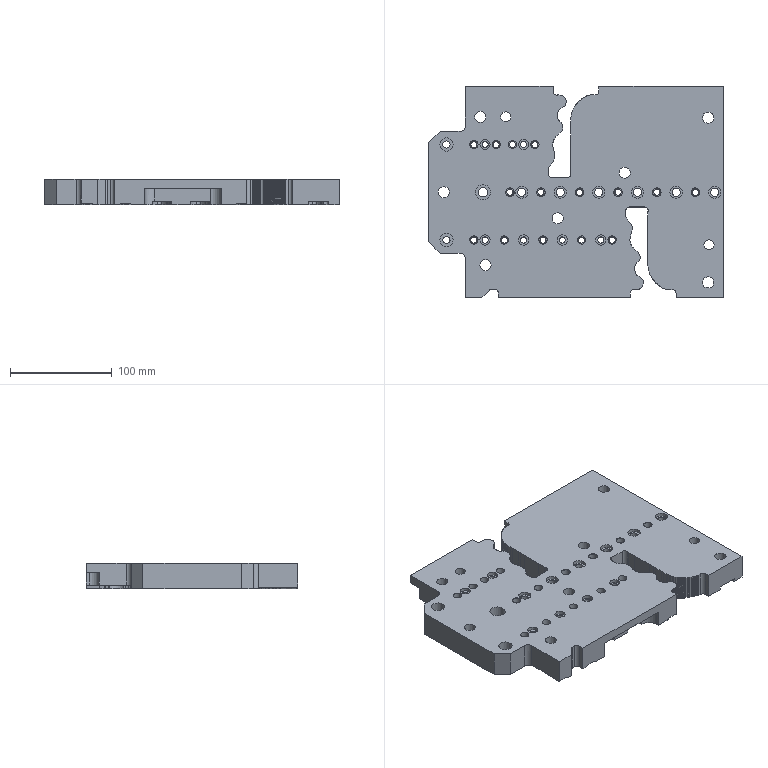Part | STEP file | PN_0034_id750_x_t | 1 solid | 797 faces | box 290 x 208 x 25 mm | volume 1200557 mm3 | plane 426 | spline 241 | cylinder 118 | sphere 6 | torus 6 | commonest cylinder face diameters 6 x29 8.2 x15 11 x13 10 x10 7 x8 14.536 x8